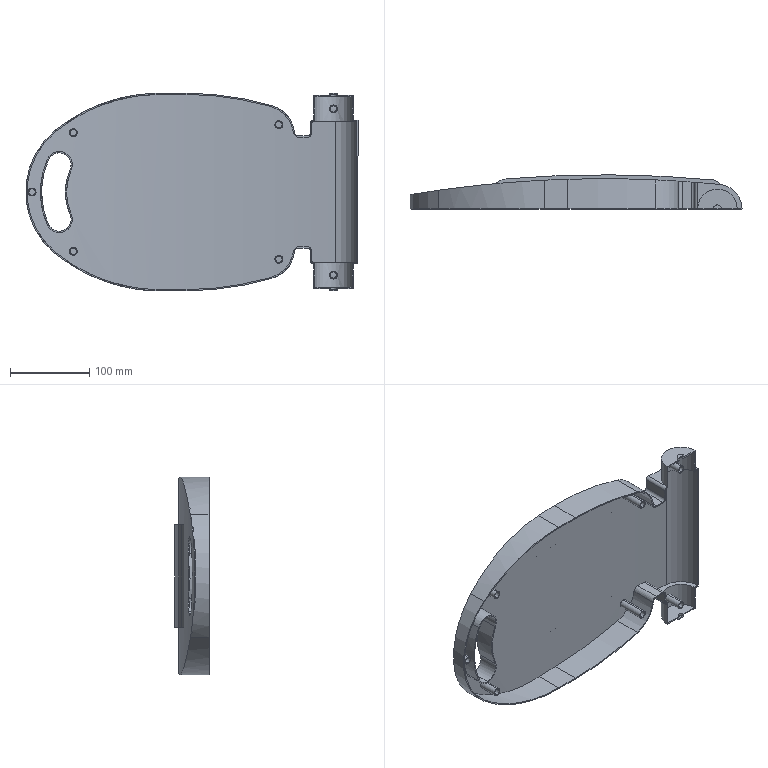Part | SolidWorks | features ICE 7, Fillet 2, CombineBodies 1, Extrusion 1, Shell 1 | 1 solid | 123 faces | box 420 x 43.06 x 250 mm | volume 378076 mm3 | cylinder 88 | plane 35 | commonest cylinder face diameters 10 x19 8 x18 2997 x6 47 x4 30 x3 33 x3